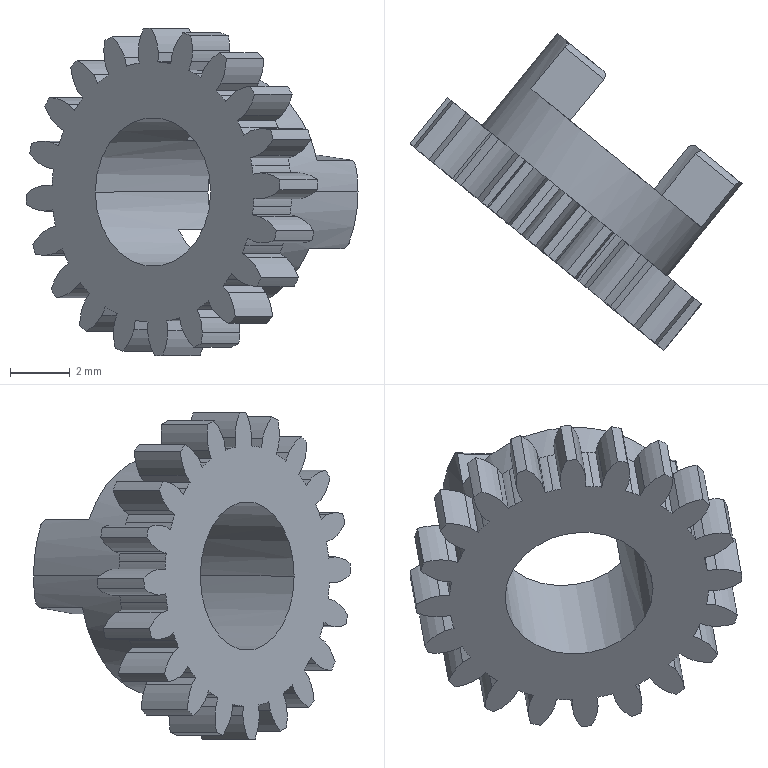Part | SolidWorks | features BaseBody 1 | 1 solid | 160 faces | box 11.156 x 10.649 x 10.999 mm | volume 194.098 mm3 | cylinder 106 | plane 50 | spline 4 | commonest cylinder face diameters 3.429 x42 4.52 x40 11 x20 5 x2 8 x2